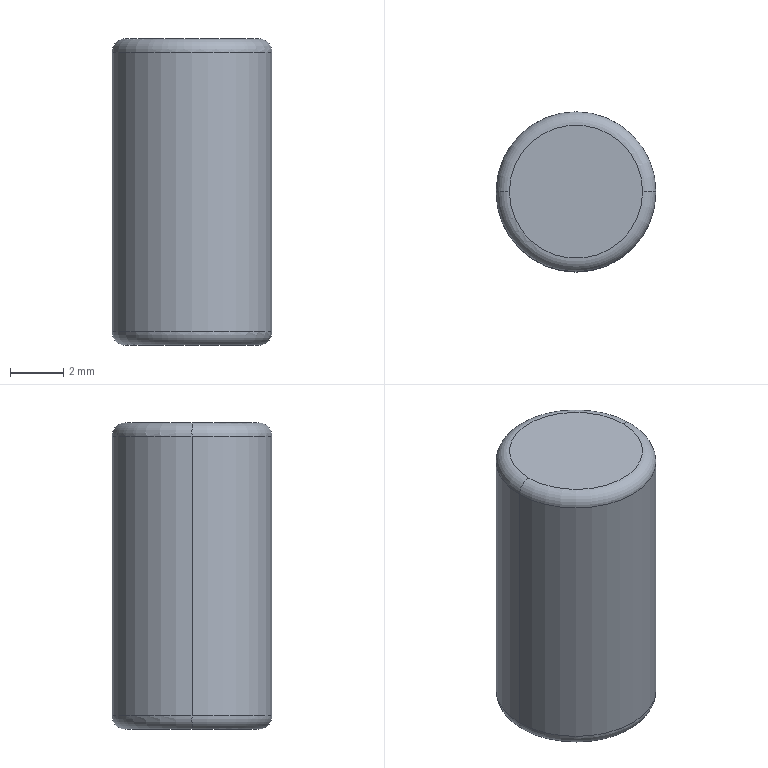Part | STEP file | 1 solid | 8 faces | box 6 x 6 x 11.5 mm | volume 323.208 mm3 | torus 4 | cylinder 2 | plane 2 | commonest cylinder face diameters 6 x2
STEP:
#1=CARTESIAN_POINT('',(0.,0.,0.));
#2=DIRECTION('',(0.,0.,1.));
#3=DIRECTION('',(1.,0.,0.));
#4=AXIS2_PLACEMENT_3D('',#1,#2,#3);
#5=CARTESIAN_POINT('',(-3.,0.,11.));
#6=VERTEX_POINT('',#5);
#7=CARTESIAN_POINT('',(3.,0.,11.));
#8=VERTEX_POINT('',#7);
#9=CARTESIAN_POINT('',(0.,0.,11.));
#10=DIRECTION('',(0.,0.,-1.));
#11=DIRECTION('',(1.,0.,0.));
#12=AXIS2_PLACEMENT_3D('',#9,#10,#11);
#13=CIRCLE('',#12,3.);
#14=CARTESIAN_POINT('',(0.,0.,11.));
#15=DIRECTION('',(0.,0.,1.));
#16=DIRECTION('',(1.,0.,0.));
#17=AXIS2_PLACEMENT_3D('',#14,#15,#16);
#18=TOROIDAL_SURFACE('',#17,2.5,0.5);
#19=CARTESIAN_POINT('',(6.283,0.));
#20=DIRECTION('',(-1.,0.));
#21=VECTOR('',#20,1.);
#22=LINE('',#19,#21);
#23=(GEOMETRIC_REPRESENTATION_CONTEXT(2)PARAMETRIC_REPRESENTATION_CONTEXT()REPRESENTATION_CONTEXT('',''));
#24=DEFINITIONAL_REPRESENTATION('',(#22),#23);
#25=PCURVE('',#18,#24);
#26=CARTESIAN_POINT('',(0.,0.,11.5));
#27=DIRECTION('',(0.,0.,-1.));
#28=DIRECTION('',(-1.,0.,0.));
#29=AXIS2_PLACEMENT_3D('',#26,#27,#28);
#30=CYLINDRICAL_SURFACE('',#29,3.);
#31=CARTESIAN_POINT('',(-3.142,0.5));
#32=DIRECTION('',(1.,0.));
#33=VECTOR('',#32,1.);
#34=LINE('',#31,#33);
#35=(GEOMETRIC_REPRESENTATION_CONTEXT(2)PARAMETRIC_REPRESENTATION_CONTEXT()REPRESENTATION_CONTEXT('',''));
#36=DEFINITIONAL_REPRESENTATION('',(#34),#35);
#37=PCURVE('',#30,#36);
#38=SURFACE_CURVE('',#13,(#25,#37),.PCURVE_S1.);
#39=EDGE_CURVE('',#6,#8,#38,.T.);
#40=ORIENTED_EDGE('',*,*,#39,.F.);
#41=CARTESIAN_POINT('',(-2.5,0.,11.5));
#42=VERTEX_POINT('',#41);
#43=CARTESIAN_POINT('',(-2.5,0.,11.));
#44=DIRECTION('',(0.,1.,0.));
#45=DIRECTION('',(-1.,0.,0.));
#46=AXIS2_PLACEMENT_3D('',#43,#44,#45);
#47=CIRCLE('',#46,0.5);
#48=CARTESIAN_POINT('',(3.142,0.));
#49=DIRECTION('',(0.,1.));
#50=VECTOR('',#49,1.);
#51=LINE('',#48,#50);
#52=(GEOMETRIC_REPRESENTATION_CONTEXT(2)PARAMETRIC_REPRESENTATION_CONTEXT()REPRESENTATION_CONTEXT('',''));
#53=DEFINITIONAL_REPRESENTATION('',(#51),#52);
#54=PCURVE('',#18,#53);
#55=CARTESIAN_POINT('',(0.,0.,11.));
#56=DIRECTION('',(0.,0.,1.));
#57=DIRECTION('',(1.,0.,0.));
#58=AXIS2_PLACEMENT_3D('',#55,#56,#57);
#59=TOROIDAL_SURFACE('',#58,2.5,0.5);
#60=CARTESIAN_POINT('',(3.142,0.));
#61=DIRECTION('',(0.,1.));
#62=VECTOR('',#61,1.);
#63=LINE('',#60,#62);
#64=(GEOMETRIC_REPRESENTATION_CONTEXT(2)PARAMETRIC_REPRESENTATION_CONTEXT()REPRESENTATION_CONTEXT('',''));
#65=DEFINITIONAL_REPRESENTATION('',(#63),#64);
#66=PCURVE('',#59,#65);
#67=SURFACE_CURVE('',#47,(#54,#66),.PCURVE_S1.);
#68=EDGE_CURVE('',#6,#42,#67,.T.);
#69=ORIENTED_EDGE('',*,*,#68,.T.);
#70=CARTESIAN_POINT('',(2.5,0.,11.5));
#71=VERTEX_POINT('',#70);
#72=CARTESIAN_POINT('',(0.,0.,11.5));
#73=DIRECTION('',(0.,0.,1.));
#74=DIRECTION('',(1.,0.,0.));
#75=AXIS2_PLACEMENT_3D('',#72,#73,#74);
#76=CIRCLE('',#75,2.5);
#77=CARTESIAN_POINT('',(0.,1.571));
#78=DIRECTION('',(1.,0.));
#79=VECTOR('',#78,1.);
#80=LINE('',#77,#79);
#81=(GEOMETRIC_REPRESENTATION_CONTEXT(2)PARAMETRIC_REPRESENTATION_CONTEXT()REPRESENTATION_CONTEXT('',''));
#82=DEFINITIONAL_REPRESENTATION('',(#80),#81);
#83=PCURVE('',#18,#82);
#84=CARTESIAN_POINT('',(0.,0.,11.5));
#85=DIRECTION('',(0.,0.,1.));
#86=DIRECTION('',(1.,0.,0.));
#87=AXIS2_PLACEMENT_3D('',#84,#85,#86);
#88=PLANE('',#87);
#89=CARTESIAN_POINT('',(0.,0.));
#90=DIRECTION('',(1.,0.));
#91=AXIS2_PLACEMENT_2D('',#89,#90);
#92=CIRCLE('',#91,2.5);
#93=(GEOMETRIC_REPRESENTATION_CONTEXT(2)PARAMETRIC_REPRESENTATION_CONTEXT()REPRESENTATION_CONTEXT('',''));
#94=DEFINITIONAL_REPRESENTATION('',(#92),#93);
#95=PCURVE('',#88,#94);
#96=SURFACE_CURVE('',#76,(#83,#95),.PCURVE_S1.);
#97=EDGE_CURVE('',#71,#42,#96,.T.);
#98=ORIENTED_EDGE('',*,*,#97,.F.);
#99=CARTESIAN_POINT('',(2.5,0.,11.));
#100=DIRECTION('',(0.,-1.,0.));
#101=DIRECTION('',(0.,0.,-1.));
#102=AXIS2_PLACEMENT_3D('',#99,#100,#101);
#103=CIRCLE('',#102,0.5);
#104=CARTESIAN_POINT('',(0.,-1.571));
#105=DIRECTION('',(0.,1.));
#106=VECTOR('',#105,1.);
#107=LINE('',#104,#106);
#108=(GEOMETRIC_REPRESENTATION_CONTEXT(2)PARAMETRIC_REPRESENTATION_CONTEXT()REPRESENTATION_CONTEXT('',''));
#109=DEFINITIONAL_REPRESENTATION('',(#107),#108);
#110=PCURVE('',#18,#109);
#111=CARTESIAN_POINT('',(6.283,-1.571));
#112=DIRECTION('',(0.,1.));
#113=VECTOR('',#112,1.);
#114=LINE('',#111,#113);
#115=(GEOMETRIC_REPRESENTATION_CONTEXT(2)PARAMETRIC_REPRESENTATION_CONTEXT()REPRESENTATION_CONTEXT('',''));
#116=DEFINITIONAL_REPRESENTATION('',(#114),#115);
#117=PCURVE('',#59,#116);
#118=SURFACE_CURVE('',#103,(#110,#117),.PCURVE_S1.);
#119=EDGE_CURVE('',#8,#71,#118,.T.);
#120=ORIENTED_EDGE('',*,*,#119,.F.);
#121=EDGE_LOOP('',(#40,#69,#98,#120));
#122=FACE_BOUND('',#121,.T.);
#123=ADVANCED_FACE('',(#122),#18,.T.);
#124=CARTESIAN_POINT('',(-2.5,0.,0.));
#125=VERTEX_POINT('',#124);
#126=CARTESIAN_POINT('',(2.5,0.,0.));
#127=VERTEX_POINT('',#126);
#128=CARTESIAN_POINT('',(0.,0.,0.));
#129=DIRECTION('',(0.,0.,-1.));
#130=DIRECTION('',(1.,0.,0.));
#131=AXIS2_PLACEMENT_3D('',#128,#129,#130);
#132=CIRCLE('',#131,2.5);
#133=CARTESIAN_POINT('',(0.,0.,0.5));
#134=DIRECTION('',(0.,0.,1.));
#135=DIRECTION('',(1.,0.,0.));
#136=AXIS2_PLACEMENT_3D('',#133,#134,#135);
#137=TOROIDAL_SURFACE('',#136,2.5,0.5);
#138=CARTESIAN_POINT('',(6.283,4.712));
#139=DIRECTION('',(-1.,0.));
#140=VECTOR('',#139,1.);
#141=LINE('',#138,#140);
#142=(GEOMETRIC_REPRESENTATION_CONTEXT(2)PARAMETRIC_REPRESENTATION_CONTEXT()REPRESENTATION_CONTEXT('',''));
#143=DEFINITIONAL_REPRESENTATION('',(#141),#142);
#144=PCURVE('',#137,#143);
#145=CARTESIAN_POINT('',(0.,0.,0.));
#146=DIRECTION('',(0.,0.,1.));
#147=DIRECTION('',(1.,0.,0.));
#148=AXIS2_PLACEMENT_3D('',#145,#146,#147);
#149=PLANE('',#148);
#150=CARTESIAN_POINT('',(2.5,0.));
#151=CARTESIAN_POINT('',(2.5,-4.33));
#152=CARTESIAN_POINT('',(-1.25,-2.165));
#153=CARTESIAN_POINT('',(-5.,0.));
#154=CARTESIAN_POINT('',(-1.25,2.165));
#155=CARTESIAN_POINT('',(2.5,4.33));
#156=CARTESIAN_POINT('',(2.5,0.));
#157=(BOUNDED_CURVE()B_SPLINE_CURVE(2,(#150,#151,#152,#153,#154,#155,#156),.UNSPECIFIED.,.T.,.F.)B_SPLINE_CURVE_WITH_KNOTS((1,2,2,2,2,1),(-2.094,0.,2.094,4.189,6.283,8.378),.UNSPECIFIED.)CURVE()GEOMETRIC_REPRESENTATION_ITEM()RATIONAL_B_SPLINE_CURVE((1.,0.5,1.,0.5,1.,0.5,1.))REPRESENTATION_ITEM(''));
#158=(GEOMETRIC_REPRESENTATION_CONTEXT(2)PARAMETRIC_REPRESENTATION_CONTEXT()REPRESENTATION_CONTEXT('',''));
#159=DEFINITIONAL_REPRESENTATION('',(#157),#158);
#160=PCURVE('',#149,#159);
#161=SURFACE_CURVE('',#132,(#144,#160),.PCURVE_S1.);
#162=EDGE_CURVE('',#125,#127,#161,.T.);
#163=ORIENTED_EDGE('',*,*,#162,.F.);
#164=CARTESIAN_POINT('',(-3.,0.,0.5));
#165=VERTEX_POINT('',#164);
#166=CARTESIAN_POINT('',(-2.5,0.,0.5));
#167=DIRECTION('',(0.,1.,0.));
#168=DIRECTION('',(-1.,0.,0.));
#169=AXIS2_PLACEMENT_3D('',#166,#167,#168);
#170=CIRCLE('',#169,0.5);
#171=CARTESIAN_POINT('',(3.142,0.));
#172=DIRECTION('',(0.,1.));
#173=VECTOR('',#172,1.);
#174=LINE('',#171,#173);
#175=(GEOMETRIC_REPRESENTATION_CONTEXT(2)PARAMETRIC_REPRESENTATION_CONTEXT()REPRESENTATION_CONTEXT('',''));
#176=DEFINITIONAL_REPRESENTATION('',(#174),#175);
#177=PCURVE('',#137,#176);
#178=CARTESIAN_POINT('',(0.,0.,0.5));
#179=DIRECTION('',(0.,0.,1.));
#180=DIRECTION('',(1.,0.,0.));
#181=AXIS2_PLACEMENT_3D('',#178,#179,#180);
#182=TOROIDAL_SURFACE('',#181,2.5,0.5);
#183=CARTESIAN_POINT('',(3.142,0.));
#184=DIRECTION('',(0.,1.));
#185=VECTOR('',#184,1.);
#186=LINE('',#183,#185);
#187=(GEOMETRIC_REPRESENTATION_CONTEXT(2)PARAMETRIC_REPRESENTATION_CONTEXT()REPRESENTATION_CONTEXT('',''));
#188=DEFINITIONAL_REPRESENTATION('',(#186),#187);
#189=PCURVE('',#182,#188);
#190=SURFACE_CURVE('',#170,(#177,#189),.PCURVE_S1.);
#191=EDGE_CURVE('',#125,#165,#190,.T.);
#192=ORIENTED_EDGE('',*,*,#191,.T.);
#193=CARTESIAN_POINT('',(3.,0.,0.5));
#194=VERTEX_POINT('',#193);
#195=CARTESIAN_POINT('',(0.,0.,0.5));
#196=DIRECTION('',(0.,0.,1.));
#197=DIRECTION('',(1.,0.,0.));
#198=AXIS2_PLACEMENT_3D('',#195,#196,#197);
#199=CIRCLE('',#198,3.);
#200=CARTESIAN_POINT('',(0.,6.283));
#201=DIRECTION('',(1.,0.));
#202=VECTOR('',#201,1.);
#203=LINE('',#200,#202);
#204=(GEOMETRIC_REPRESENTATION_CONTEXT(2)PARAMETRIC_REPRESENTATION_CONTEXT()REPRESENTATION_CONTEXT('',''));
#205=DEFINITIONAL_REPRESENTATION('',(#203),#204);
#206=PCURVE('',#137,#205);
#207=CARTESIAN_POINT('',(3.142,11.));
#208=DIRECTION('',(-1.,0.));
#209=VECTOR('',#208,1.);
#210=LINE('',#207,#209);
#211=(GEOMETRIC_REPRESENTATION_CONTEXT(2)PARAMETRIC_REPRESENTATION_CONTEXT()REPRESENTATION_CONTEXT('',''));
#212=DEFINITIONAL_REPRESENTATION('',(#210),#211);
#213=PCURVE('',#30,#212);
#214=SURFACE_CURVE('',#199,(#206,#213),.PCURVE_S1.);
#215=EDGE_CURVE('',#194,#165,#214,.T.);
#216=ORIENTED_EDGE('',*,*,#215,.F.);
#217=CARTESIAN_POINT('',(2.5,0.,0.5));
#218=DIRECTION('',(0.,-1.,0.));
#219=DIRECTION('',(0.,0.,-1.));
#220=AXIS2_PLACEMENT_3D('',#217,#218,#219);
#221=CIRCLE('',#220,0.5);
#222=CARTESIAN_POINT('',(0.,4.712));
#223=DIRECTION('',(0.,1.));
#224=VECTOR('',#223,1.);
#225=LINE('',#222,#224);
#226=(GEOMETRIC_REPRESENTATION_CONTEXT(2)PARAMETRIC_REPRESENTATION_CONTEXT()REPRESENTATION_CONTEXT('',''));
#227=DEFINITIONAL_REPRESENTATION('',(#225),#226);
#228=PCURVE('',#137,#227);
#229=CARTESIAN_POINT('',(6.283,4.712));
#230=DIRECTION('',(0.,1.));
#231=VECTOR('',#230,1.);
#232=LINE('',#229,#231);
#233=(GEOMETRIC_REPRESENTATION_CONTEXT(2)PARAMETRIC_REPRESENTATION_CONTEXT()REPRESENTATION_CONTEXT('',''));
#234=DEFINITIONAL_REPRESENTATION('',(#232),#233);
#235=PCURVE('',#182,#234);
#236=SURFACE_CURVE('',#221,(#228,#235),.PCURVE_S1.);
#237=EDGE_CURVE('',#127,#194,#236,.T.);
#238=ORIENTED_EDGE('',*,*,#237,.F.);
#239=EDGE_LOOP('',(#163,#192,#216,#238));
#240=FACE_BOUND('',#239,.T.);
#241=ADVANCED_FACE('',(#240),#137,.T.);
#242=ORIENTED_EDGE('',*,*,#39,.T.);
#243=CARTESIAN_POINT('',(3.,0.,11.5));
#244=DIRECTION('',(0.,0.,-1.));
#245=VECTOR('',#244,1.);
#246=LINE('',#243,#245);
#247=CARTESIAN_POINT('',(3.142,0.));
#248=DIRECTION('',(0.,1.));
#249=VECTOR('',#248,1.);
#250=LINE('',#247,#249);
#251=(GEOMETRIC_REPRESENTATION_CONTEXT(2)PARAMETRIC_REPRESENTATION_CONTEXT()REPRESENTATION_CONTEXT('',''));
#252=DEFINITIONAL_REPRESENTATION('',(#250),#251);
#253=PCURVE('',#30,#252);
#254=CARTESIAN_POINT('',(0.,0.,11.5));
#255=DIRECTION('',(0.,0.,-1.));
#256=DIRECTION('',(-1.,0.,0.));
#257=AXIS2_PLACEMENT_3D('',#254,#255,#256);
#258=CYLINDRICAL_SURFACE('',#257,3.);
#259=CARTESIAN_POINT('',(3.142,0.));
#260=DIRECTION('',(0.,1.));
#261=VECTOR('',#260,1.);
#262=LINE('',#259,#261);
#263=(GEOMETRIC_REPRESENTATION_CONTEXT(2)PARAMETRIC_REPRESENTATION_CONTEXT()REPRESENTATION_CONTEXT('',''));
#264=DEFINITIONAL_REPRESENTATION('',(#262),#263);
#265=PCURVE('',#258,#264);
#266=SURFACE_CURVE('',#246,(#253,#265),.PCURVE_S1.);
#267=EDGE_CURVE('',#8,#194,#266,.T.);
#268=ORIENTED_EDGE('',*,*,#267,.T.);
#269=ORIENTED_EDGE('',*,*,#215,.T.);
#270=CARTESIAN_POINT('',(-3.,0.,11.5));
#271=DIRECTION('',(0.,0.,-1.));
#272=VECTOR('',#271,1.);
#273=LINE('',#270,#272);
#274=CARTESIAN_POINT('',(0.,0.));
#275=DIRECTION('',(0.,1.));
#276=VECTOR('',#275,1.);
#277=LINE('',#274,#276);
#278=(GEOMETRIC_REPRESENTATION_CONTEXT(2)PARAMETRIC_REPRESENTATION_CONTEXT()REPRESENTATION_CONTEXT('',''));
#279=DEFINITIONAL_REPRESENTATION('',(#277),#278);
#280=PCURVE('',#30,#279);
#281=CARTESIAN_POINT('',(6.283,0.));
#282=DIRECTION('',(0.,1.));
#283=VECTOR('',#282,1.);
#284=LINE('',#281,#283);
#285=(GEOMETRIC_REPRESENTATION_CONTEXT(2)PARAMETRIC_REPRESENTATION_CONTEXT()REPRESENTATION_CONTEXT('',''));
#286=DEFINITIONAL_REPRESENTATION('',(#284),#285);
#287=PCURVE('',#258,#286);
#288=SURFACE_CURVE('',#273,(#280,#287),.PCURVE_S1.);
#289=EDGE_CURVE('',#6,#165,#288,.T.);
#290=ORIENTED_EDGE('',*,*,#289,.F.);
#291=EDGE_LOOP('',(#242,#268,#269,#290));
#292=FACE_BOUND('',#291,.T.);
#293=ADVANCED_FACE('',(#292),#30,.T.);
#294=ORIENTED_EDGE('',*,*,#267,.F.);
#295=CARTESIAN_POINT('',(0.,0.,11.));
#296=DIRECTION('',(0.,0.,-1.));
#297=DIRECTION('',(1.,0.,0.));
#298=AXIS2_PLACEMENT_3D('',#295,#296,#297);
#299=CIRCLE('',#298,3.);
#300=CARTESIAN_POINT('',(3.142,0.5));
#301=DIRECTION('',(1.,0.));
#302=VECTOR('',#301,1.);
#303=LINE('',#300,#302);
#304=(GEOMETRIC_REPRESENTATION_CONTEXT(2)PARAMETRIC_REPRESENTATION_CONTEXT()REPRESENTATION_CONTEXT('',''));
#305=DEFINITIONAL_REPRESENTATION('',(#303),#304);
#306=PCURVE('',#258,#305);
#307=CARTESIAN_POINT('',(6.283,0.));
#308=DIRECTION('',(-1.,0.));
#309=VECTOR('',#308,1.);
#310=LINE('',#307,#309);
#311=(GEOMETRIC_REPRESENTATION_CONTEXT(2)PARAMETRIC_REPRESENTATION_CONTEXT()REPRESENTATION_CONTEXT('',''));
#312=DEFINITIONAL_REPRESENTATION('',(#310),#311);
#313=PCURVE('',#59,#312);
#314=SURFACE_CURVE('',#299,(#306,#313),.PCURVE_S1.);
#315=EDGE_CURVE('',#8,#6,#314,.T.);
#316=ORIENTED_EDGE('',*,*,#315,.T.);
#317=ORIENTED_EDGE('',*,*,#289,.T.);
#318=CARTESIAN_POINT('',(0.,0.,0.5));
#319=DIRECTION('',(0.,0.,1.));
#320=DIRECTION('',(1.,0.,0.));
#321=AXIS2_PLACEMENT_3D('',#318,#319,#320);
#322=CIRCLE('',#321,3.);
#323=CARTESIAN_POINT('',(9.425,11.));
#324=DIRECTION('',(-1.,0.));
#325=VECTOR('',#324,1.);
#326=LINE('',#323,#325);
#327=(GEOMETRIC_REPRESENTATION_CONTEXT(2)PARAMETRIC_REPRESENTATION_CONTEXT()REPRESENTATION_CONTEXT('',''));
#328=DEFINITIONAL_REPRESENTATION('',(#326),#327);
#329=PCURVE('',#258,#328);
#330=CARTESIAN_POINT('',(0.,6.283));
#331=DIRECTION('',(1.,0.));
#332=VECTOR('',#331,1.);
#333=LINE('',#330,#332);
#334=(GEOMETRIC_REPRESENTATION_CONTEXT(2)PARAMETRIC_REPRESENTATION_CONTEXT()REPRESENTATION_CONTEXT('',''));
#335=DEFINITIONAL_REPRESENTATION('',(#333),#334);
#336=PCURVE('',#182,#335);
#337=SURFACE_CURVE('',#322,(#329,#336),.PCURVE_S1.);
#338=EDGE_CURVE('',#165,#194,#337,.T.);
#339=ORIENTED_EDGE('',*,*,#338,.T.);
#340=EDGE_LOOP('',(#294,#316,#317,#339));
#341=FACE_BOUND('',#340,.T.);
#342=ADVANCED_FACE('',(#341),#258,.T.);
#343=ORIENTED_EDGE('',*,*,#97,.T.);
#344=CARTESIAN_POINT('',(0.,0.,11.5));
#345=DIRECTION('',(0.,0.,1.));
#346=DIRECTION('',(1.,0.,0.));
#347=AXIS2_PLACEMENT_3D('',#344,#345,#346);
#348=CIRCLE('',#347,2.5);
#349=CARTESIAN_POINT('',(0.,0.));
#350=DIRECTION('',(1.,0.));
#351=AXIS2_PLACEMENT_2D('',#349,#350);
#352=CIRCLE('',#351,2.5);
#353=(GEOMETRIC_REPRESENTATION_CONTEXT(2)PARAMETRIC_REPRESENTATION_CONTEXT()REPRESENTATION_CONTEXT('',''));
#354=DEFINITIONAL_REPRESENTATION('',(#352),#353);
#355=PCURVE('',#88,#354);
#356=CARTESIAN_POINT('',(0.,1.571));
#357=DIRECTION('',(1.,0.));
#358=VECTOR('',#357,1.);
#359=LINE('',#356,#358);
#360=(GEOMETRIC_REPRESENTATION_CONTEXT(2)PARAMETRIC_REPRESENTATION_CONTEXT()REPRESENTATION_CONTEXT('',''));
#361=DEFINITIONAL_REPRESENTATION('',(#359),#360);
#362=PCURVE('',#59,#361);
#363=SURFACE_CURVE('',#348,(#355,#362),.PCURVE_S1.);
#364=EDGE_CURVE('',#42,#71,#363,.T.);
#365=ORIENTED_EDGE('',*,*,#364,.T.);
#366=EDGE_LOOP('',(#343,#365));
#367=FACE_BOUND('',#366,.T.);
#368=ADVANCED_FACE('',(#367),#88,.T.);
#369=CARTESIAN_POINT('',(0.,0.,0.));
#370=DIRECTION('',(0.,0.,-1.));
#371=DIRECTION('',(1.,0.,0.));
#372=AXIS2_PLACEMENT_3D('',#369,#370,#371);
#373=CIRCLE('',#372,2.5);
#374=CARTESIAN_POINT('',(2.5,0.));
#375=CARTESIAN_POINT('',(2.5,-4.33));
#376=CARTESIAN_POINT('',(-1.25,-2.165));
#377=CARTESIAN_POINT('',(-5.,0.));
#378=CARTESIAN_POINT('',(-1.25,2.165));
#379=CARTESIAN_POINT('',(2.5,4.33));
#380=CARTESIAN_POINT('',(2.5,0.));
#381=(BOUNDED_CURVE()B_SPLINE_CURVE(2,(#374,#375,#376,#377,#378,#379,#380),.UNSPECIFIED.,.T.,.F.)B_SPLINE_CURVE_WITH_KNOTS((1,2,2,2,2,1),(-2.094,0.,2.094,4.189,6.283,8.378),.UNSPECIFIED.)CURVE()GEOMETRIC_REPRESENTATION_ITEM()RATIONAL_B_SPLINE_CURVE((1.,0.5,1.,0.5,1.,0.5,1.))REPRESENTATION_ITEM(''));
#382=(GEOMETRIC_REPRESENTATION_CONTEXT(2)PARAMETRIC_REPRESENTATION_CONTEXT()REPRESENTATION_CONTEXT('',''));
#383=DEFINITIONAL_REPRESENTATION('',(#381),#382);
#384=PCURVE('',#149,#383);
#385=CARTESIAN_POINT('',(6.283,4.712));
#386=DIRECTION('',(-1.,0.));
#387=VECTOR('',#386,1.);
#388=LINE('',#385,#387);
#389=(GEOMETRIC_REPRESENTATION_CONTEXT(2)PARAMETRIC_REPRESENTATION_CONTEXT()REPRESENTATION_CONTEXT('',''));
#390=DEFINITIONAL_REPRESENTATION('',(#388),#389);
#391=PCURVE('',#182,#390);
#392=SURFACE_CURVE('',#373,(#384,#391),.PCURVE_S1.);
#393=EDGE_CURVE('',#127,#125,#392,.T.);
#394=ORIENTED_EDGE('',*,*,#393,.T.);
#395=ORIENTED_EDGE('',*,*,#162,.T.);
#396=EDGE_LOOP('',(#394,#395));
#397=FACE_BOUND('',#396,.T.);
#398=ADVANCED_FACE('',(#397),#149,.F.);
#399=ORIENTED_EDGE('',*,*,#191,.F.);
#400=ORIENTED_EDGE('',*,*,#393,.F.);
#401=ORIENTED_EDGE('',*,*,#237,.T.);
#402=ORIENTED_EDGE('',*,*,#338,.F.);
#403=EDGE_LOOP('',(#399,#400,#401,#402));
#404=FACE_BOUND('',#403,.T.);
#405=ADVANCED_FACE('',(#404),#182,.T.);
#406=ORIENTED_EDGE('',*,*,#68,.F.);
#407=ORIENTED_EDGE('',*,*,#315,.F.);
#408=ORIENTED_EDGE('',*,*,#119,.T.);
#409=ORIENTED_EDGE('',*,*,#364,.F.);
#410=EDGE_LOOP('',(#406,#407,#408,#409));
#411=FACE_BOUND('',#410,.T.);
#412=ADVANCED_FACE('',(#411),#59,.T.);
#413=CLOSED_SHELL('',(#123,#241,#293,#342,#368,#398,#405,#412));
#414=MANIFOLD_SOLID_BREP('',#413);
#415=(LENGTH_UNIT()NAMED_UNIT(*)SI_UNIT(.MILLI.,.METRE.));
#416=UNCERTAINTY_MEASURE_WITH_UNIT(LENGTH_MEASURE(0.0000001),#415,'','');
#417=(NAMED_UNIT(*)PLANE_ANGLE_UNIT()SI_UNIT($,.RADIAN.));
#418=(NAMED_UNIT(*)SI_UNIT($,.STERADIAN.)SOLID_ANGLE_UNIT());
#419=(GEOMETRIC_REPRESENTATION_CONTEXT(3)GLOBAL_UNCERTAINTY_ASSIGNED_CONTEXT((#416))GLOBAL_UNIT_ASSIGNED_CONTEXT((#415,#417,#418))REPRESENTATION_CONTEXT('',''));
#420=ADVANCED_BREP_SHAPE_REPRESENTATION('',(#4,#414),#419);